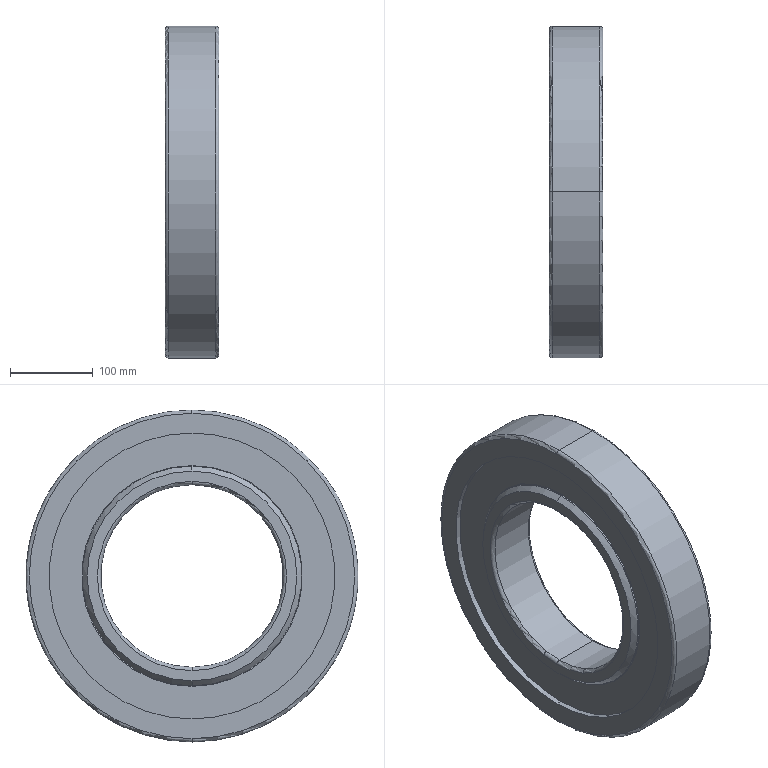Part | SolidWorks | features Revolution 5, Attribute 2, CirPattern 1, RefAxis 1 | 1 solid | 44 faces | box 65 x 400 x 400 mm | volume 5037424 mm3 | torus 16 | cylinder 16 | plane 8 | cone 4 | commonest cylinder face diameters 264.1 x4 344.425 x4 355.9 x4 220 x2 400 x2
STEP:
#1=CARTESIAN_POINT('',(32.5,0.,-126.312));
#2=VERTEX_POINT('',#1);
#3=CARTESIAN_POINT('',(32.5,0.,126.312));
#4=VERTEX_POINT('',#3);
#5=CARTESIAN_POINT('',(32.5,0.,0.));
#6=DIRECTION('',(1.,0.,0.));
#7=DIRECTION('',(0.,0.,-1.));
#8=AXIS2_PLACEMENT_3D('',#5,#6,#7);
#9=CIRCLE('',#8,126.313);
#10=EDGE_CURVE('',#2,#4,#9,.T.);
#11=ORIENTED_EDGE('',*,*,#10,.F.);
#12=CARTESIAN_POINT('',(26.,0.,-132.05));
#13=VERTEX_POINT('',#12);
#14=CARTESIAN_POINT('',(32.5,0.,-126.313));
#15=DIRECTION('',(-0.7497,0.,-0.6618));
#16=VECTOR('',#15,1000.);
#17=LINE('',#14,#16);
#18=EDGE_CURVE('',#2,#13,#17,.T.);
#19=ORIENTED_EDGE('',*,*,#18,.T.);
#20=CARTESIAN_POINT('',(26.,0.,132.05));
#21=VERTEX_POINT('',#20);
#22=CARTESIAN_POINT('',(26.,0.,0.));
#23=DIRECTION('',(1.,0.,0.));
#24=DIRECTION('',(0.,0.,-1.));
#25=AXIS2_PLACEMENT_3D('',#22,#23,#24);
#26=CIRCLE('',#25,132.05);
#27=EDGE_CURVE('',#13,#21,#26,.T.);
#28=ORIENTED_EDGE('',*,*,#27,.T.);
#29=CARTESIAN_POINT('',(32.5,0.,126.313));
#30=DIRECTION('',(-0.7497,0.,0.6618));
#31=VECTOR('',#30,1000.);
#32=LINE('',#29,#31);
#33=EDGE_CURVE('',#4,#21,#32,.T.);
#34=ORIENTED_EDGE('',*,*,#33,.F.);
#35=EDGE_LOOP('',(#11,#19,#28,#34));
#36=FACE_OUTER_BOUND('',#35,.T.);
#37=CARTESIAN_POINT('',(32.5,0.,0.));
#38=DIRECTION('',(-1.,0.,0.));
#39=DIRECTION('',(0.,0.,1.));
#40=AXIS2_PLACEMENT_3D('',#37,#38,#39);
#41=CONICAL_SURFACE('',#40,126.313,0.7232);
#42=ADVANCED_FACE('',(#36),#41,.T.);
#43=CARTESIAN_POINT('',(32.5,0.,-114.));
#44=VERTEX_POINT('',#43);
#45=CARTESIAN_POINT('',(32.5,0.,114.));
#46=VERTEX_POINT('',#45);
#47=CARTESIAN_POINT('',(32.5,0.,0.));
#48=DIRECTION('',(1.,0.,0.));
#49=DIRECTION('',(0.,0.,-1.));
#50=AXIS2_PLACEMENT_3D('',#47,#48,#49);
#51=CIRCLE('',#50,114.);
#52=EDGE_CURVE('',#44,#46,#51,.T.);
#53=ORIENTED_EDGE('',*,*,#52,.T.);
#54=CARTESIAN_POINT('',(28.5,0.,110.));
#55=VERTEX_POINT('',#54);
#56=CARTESIAN_POINT('',(28.5,0.,114.));
#57=DIRECTION('',(0.,1.,0.));
#58=DIRECTION('',(0.,0.,1.));
#59=AXIS2_PLACEMENT_3D('',#56,#57,#58);
#60=CIRCLE('',#59,4.);
#61=EDGE_CURVE('',#46,#55,#60,.T.);
#62=ORIENTED_EDGE('',*,*,#61,.T.);
#63=CARTESIAN_POINT('',(28.5,0.,-110.));
#64=VERTEX_POINT('',#63);
#65=CARTESIAN_POINT('',(28.5,0.,0.));
#66=DIRECTION('',(1.,0.,0.));
#67=DIRECTION('',(0.,0.,-1.));
#68=AXIS2_PLACEMENT_3D('',#65,#66,#67);
#69=CIRCLE('',#68,110.);
#70=EDGE_CURVE('',#64,#55,#69,.T.);
#71=ORIENTED_EDGE('',*,*,#70,.F.);
#72=CARTESIAN_POINT('',(28.5,0.,-114.));
#73=DIRECTION('',(0.,-1.,0.));
#74=DIRECTION('',(0.,0.,-1.));
#75=AXIS2_PLACEMENT_3D('',#72,#73,#74);
#76=CIRCLE('',#75,4.);
#77=EDGE_CURVE('',#44,#64,#76,.T.);
#78=ORIENTED_EDGE('',*,*,#77,.F.);
#79=EDGE_LOOP('',(#53,#62,#71,#78));
#80=FACE_OUTER_BOUND('',#79,.T.);
#81=CARTESIAN_POINT('',(28.5,0.,0.));
#82=DIRECTION('',(1.,0.,0.));
#83=DIRECTION('',(0.,0.,-1.));
#84=AXIS2_PLACEMENT_3D('',#81,#82,#83);
#85=TOROIDAL_SURFACE('',#84,114.,4.);
#86=ADVANCED_FACE('',(#80),#85,.T.);
#87=CARTESIAN_POINT('',(-28.5,0.,110.));
#88=VERTEX_POINT('',#87);
#89=CARTESIAN_POINT('',(-28.5,0.,-110.));
#90=VERTEX_POINT('',#89);
#91=CARTESIAN_POINT('',(-28.5,0.,0.));
#92=DIRECTION('',(1.,0.,0.));
#93=DIRECTION('',(0.,0.,-1.));
#94=AXIS2_PLACEMENT_3D('',#91,#92,#93);
#95=CIRCLE('',#94,110.);
#96=EDGE_CURVE('',#88,#90,#95,.T.);
#97=ORIENTED_EDGE('',*,*,#96,.F.);
#98=CARTESIAN_POINT('',(-90.,0.,110.));
#99=DIRECTION('',(1.,0.,0.));
#100=VECTOR('',#99,1000.);
#101=LINE('',#98,#100);
#102=EDGE_CURVE('',#88,#55,#101,.T.);
#103=ORIENTED_EDGE('',*,*,#102,.T.);
#104=CARTESIAN_POINT('',(28.5,0.,0.));
#105=DIRECTION('',(1.,0.,0.));
#106=DIRECTION('',(0.,0.,-1.));
#107=AXIS2_PLACEMENT_3D('',#104,#105,#106);
#108=CIRCLE('',#107,110.);
#109=EDGE_CURVE('',#55,#64,#108,.T.);
#110=ORIENTED_EDGE('',*,*,#109,.T.);
#111=CARTESIAN_POINT('',(-90.,0.,-110.));
#112=DIRECTION('',(1.,0.,0.));
#113=VECTOR('',#112,1000.);
#114=LINE('',#111,#113);
#115=EDGE_CURVE('',#90,#64,#114,.T.);
#116=ORIENTED_EDGE('',*,*,#115,.F.);
#117=EDGE_LOOP('',(#97,#103,#110,#116));
#118=FACE_OUTER_BOUND('',#117,.T.);
#119=CARTESIAN_POINT('',(-90.,0.,0.));
#120=DIRECTION('',(1.,0.,0.));
#121=DIRECTION('',(0.,0.,-1.));
#122=AXIS2_PLACEMENT_3D('',#119,#120,#121);
#123=CYLINDRICAL_SURFACE('',#122,110.);
#124=ADVANCED_FACE('',(#118),#123,.F.);
#125=CARTESIAN_POINT('',(-28.5,0.,0.));
#126=DIRECTION('',(1.,0.,0.));
#127=DIRECTION('',(0.,0.,-1.));
#128=AXIS2_PLACEMENT_3D('',#125,#126,#127);
#129=CIRCLE('',#128,110.);
#130=EDGE_CURVE('',#90,#88,#129,.T.);
#131=ORIENTED_EDGE('',*,*,#130,.T.);
#132=CARTESIAN_POINT('',(-32.5,0.,114.));
#133=VERTEX_POINT('',#132);
#134=CARTESIAN_POINT('',(-28.5,0.,114.));
#135=DIRECTION('',(0.,1.,0.));
#136=DIRECTION('',(0.,0.,1.));
#137=AXIS2_PLACEMENT_3D('',#134,#135,#136);
#138=CIRCLE('',#137,4.);
#139=EDGE_CURVE('',#88,#133,#138,.T.);
#140=ORIENTED_EDGE('',*,*,#139,.T.);
#141=CARTESIAN_POINT('',(-32.5,0.,-114.));
#142=VERTEX_POINT('',#141);
#143=CARTESIAN_POINT('',(-32.5,0.,0.));
#144=DIRECTION('',(1.,0.,0.));
#145=DIRECTION('',(0.,0.,-1.));
#146=AXIS2_PLACEMENT_3D('',#143,#144,#145);
#147=CIRCLE('',#146,114.);
#148=EDGE_CURVE('',#142,#133,#147,.T.);
#149=ORIENTED_EDGE('',*,*,#148,.F.);
#150=CARTESIAN_POINT('',(-28.5,0.,-114.));
#151=DIRECTION('',(0.,-1.,0.));
#152=DIRECTION('',(0.,0.,-1.));
#153=AXIS2_PLACEMENT_3D('',#150,#151,#152);
#154=CIRCLE('',#153,4.);
#155=EDGE_CURVE('',#90,#142,#154,.T.);
#156=ORIENTED_EDGE('',*,*,#155,.F.);
#157=EDGE_LOOP('',(#131,#140,#149,#156));
#158=FACE_OUTER_BOUND('',#157,.T.);
#159=CARTESIAN_POINT('',(-28.5,0.,0.));
#160=DIRECTION('',(1.,0.,0.));
#161=DIRECTION('',(0.,0.,-1.));
#162=AXIS2_PLACEMENT_3D('',#159,#160,#161);
#163=TOROIDAL_SURFACE('',#162,114.,4.);
#164=ADVANCED_FACE('',(#158),#163,.T.);
#165=CARTESIAN_POINT('',(-32.5,0.,-126.313));
#166=VERTEX_POINT('',#165);
#167=CARTESIAN_POINT('',(-32.5,0.,126.312));
#168=VERTEX_POINT('',#167);
#169=CARTESIAN_POINT('',(-32.5,0.,0.));
#170=DIRECTION('',(1.,0.,0.));
#171=DIRECTION('',(0.,0.,-1.));
#172=AXIS2_PLACEMENT_3D('',#169,#170,#171);
#173=CIRCLE('',#172,126.313);
#174=EDGE_CURVE('',#166,#168,#173,.T.);
#175=ORIENTED_EDGE('',*,*,#174,.T.);
#176=CARTESIAN_POINT('',(-26.,0.,132.05));
#177=VERTEX_POINT('',#176);
#178=CARTESIAN_POINT('',(-26.,0.,132.05));
#179=DIRECTION('',(0.7497,0.,0.6618));
#180=VECTOR('',#179,1000.);
#181=LINE('',#178,#180);
#182=EDGE_CURVE('',#168,#177,#181,.T.);
#183=ORIENTED_EDGE('',*,*,#182,.T.);
#184=CARTESIAN_POINT('',(-26.,0.,-132.05));
#185=VERTEX_POINT('',#184);
#186=CARTESIAN_POINT('',(-26.,0.,0.));
#187=DIRECTION('',(1.,0.,0.));
#188=DIRECTION('',(0.,0.,-1.));
#189=AXIS2_PLACEMENT_3D('',#186,#187,#188);
#190=CIRCLE('',#189,132.05);
#191=EDGE_CURVE('',#185,#177,#190,.T.);
#192=ORIENTED_EDGE('',*,*,#191,.F.);
#193=CARTESIAN_POINT('',(-26.,0.,-132.05));
#194=DIRECTION('',(0.7497,0.,-0.6618));
#195=VECTOR('',#194,1000.);
#196=LINE('',#193,#195);
#197=EDGE_CURVE('',#166,#185,#196,.T.);
#198=ORIENTED_EDGE('',*,*,#197,.F.);
#199=EDGE_LOOP('',(#175,#183,#192,#198));
#200=FACE_OUTER_BOUND('',#199,.T.);
#201=CARTESIAN_POINT('',(-26.,0.,0.));
#202=DIRECTION('',(1.,0.,0.));
#203=DIRECTION('',(0.,0.,-1.));
#204=AXIS2_PLACEMENT_3D('',#201,#202,#203);
#205=CONICAL_SURFACE('',#204,132.05,0.7232);
#206=ADVANCED_FACE('',(#200),#205,.T.);
#207=CARTESIAN_POINT('',(23.877,0.,-132.05));
#208=VERTEX_POINT('',#207);
#209=CARTESIAN_POINT('',(23.877,0.,132.05));
#210=VERTEX_POINT('',#209);
#211=CARTESIAN_POINT('',(23.877,0.,0.));
#212=DIRECTION('',(1.,0.,0.));
#213=DIRECTION('',(0.,0.,1.));
#214=AXIS2_PLACEMENT_3D('',#211,#212,#213);
#215=CIRCLE('',#214,132.05);
#216=EDGE_CURVE('',#208,#210,#215,.T.);
#217=ORIENTED_EDGE('',*,*,#216,.T.);
#218=CARTESIAN_POINT('',(-90.,0.,132.05));
#219=DIRECTION('',(1.,0.,0.));
#220=VECTOR('',#219,1000.);
#221=LINE('',#218,#220);
#222=EDGE_CURVE('',#210,#21,#221,.T.);
#223=ORIENTED_EDGE('',*,*,#222,.T.);
#224=ORIENTED_EDGE('',*,*,#27,.F.);
#225=CARTESIAN_POINT('',(-90.,0.,-132.05));
#226=DIRECTION('',(1.,0.,0.));
#227=VECTOR('',#226,1000.);
#228=LINE('',#225,#227);
#229=EDGE_CURVE('',#208,#13,#228,.T.);
#230=ORIENTED_EDGE('',*,*,#229,.F.);
#231=EDGE_LOOP('',(#217,#223,#224,#230));
#232=FACE_OUTER_BOUND('',#231,.T.);
#233=CARTESIAN_POINT('',(-90.,0.,0.));
#234=DIRECTION('',(1.,0.,0.));
#235=DIRECTION('',(0.,0.,-1.));
#236=AXIS2_PLACEMENT_3D('',#233,#234,#235);
#237=CYLINDRICAL_SURFACE('',#236,132.05);
#238=ADVANCED_FACE('',(#232),#237,.T.);
#239=ORIENTED_EDGE('',*,*,#191,.T.);
#240=CARTESIAN_POINT('',(-23.877,0.,132.05));
#241=VERTEX_POINT('',#240);
#242=CARTESIAN_POINT('',(-90.,0.,132.05));
#243=DIRECTION('',(1.,0.,0.));
#244=VECTOR('',#243,1000.);
#245=LINE('',#242,#244);
#246=EDGE_CURVE('',#177,#241,#245,.T.);
#247=ORIENTED_EDGE('',*,*,#246,.T.);
#248=CARTESIAN_POINT('',(-23.877,0.,-132.05));
#249=VERTEX_POINT('',#248);
#250=CARTESIAN_POINT('',(-23.877,0.,0.));
#251=DIRECTION('',(-1.,0.,0.));
#252=DIRECTION('',(0.,0.,-1.));
#253=AXIS2_PLACEMENT_3D('',#250,#251,#252);
#254=CIRCLE('',#253,132.05);
#255=EDGE_CURVE('',#241,#249,#254,.T.);
#256=ORIENTED_EDGE('',*,*,#255,.T.);
#257=CARTESIAN_POINT('',(-90.,0.,-132.05));
#258=DIRECTION('',(1.,0.,0.));
#259=VECTOR('',#258,1000.);
#260=LINE('',#257,#259);
#261=EDGE_CURVE('',#185,#249,#260,.T.);
#262=ORIENTED_EDGE('',*,*,#261,.F.);
#263=EDGE_LOOP('',(#239,#247,#256,#262));
#264=FACE_OUTER_BOUND('',#263,.T.);
#265=CARTESIAN_POINT('',(-90.,0.,0.));
#266=DIRECTION('',(1.,0.,0.));
#267=DIRECTION('',(0.,0.,-1.));
#268=AXIS2_PLACEMENT_3D('',#265,#266,#267);
#269=CYLINDRICAL_SURFACE('',#268,132.05);
#270=ADVANCED_FACE('',(#264),#269,.T.);
#271=CARTESIAN_POINT('',(23.877,0.,-177.95));
#272=VERTEX_POINT('',#271);
#273=CARTESIAN_POINT('',(23.877,0.,177.95));
#274=VERTEX_POINT('',#273);
#275=CARTESIAN_POINT('',(23.877,0.,0.));
#276=DIRECTION('',(1.,0.,0.));
#277=DIRECTION('',(0.,0.,1.));
#278=AXIS2_PLACEMENT_3D('',#275,#276,#277);
#279=CIRCLE('',#278,177.95);
#280=EDGE_CURVE('',#272,#274,#279,.T.);
#281=ORIENTED_EDGE('',*,*,#280,.T.);
#282=CARTESIAN_POINT('',(24.7,0.,177.037));
#283=VERTEX_POINT('',#282);
#284=CARTESIAN_POINT('',(23.782,0.,177.037));
#285=DIRECTION('',(0.,1.,0.));
#286=DIRECTION('',(0.,0.,1.));
#287=AXIS2_PLACEMENT_3D('',#284,#285,#286);
#288=CIRCLE('',#287,0.9182);
#289=EDGE_CURVE('',#274,#283,#288,.T.);
#290=ORIENTED_EDGE('',*,*,#289,.T.);
#291=CARTESIAN_POINT('',(24.7,0.,-177.037));
#292=VERTEX_POINT('',#291);
#293=CARTESIAN_POINT('',(24.7,0.,0.));
#294=DIRECTION('',(1.,0.,0.));
#295=DIRECTION('',(0.,0.,-1.));
#296=AXIS2_PLACEMENT_3D('',#293,#294,#295);
#297=CIRCLE('',#296,177.037);
#298=EDGE_CURVE('',#292,#283,#297,.T.);
#299=ORIENTED_EDGE('',*,*,#298,.F.);
#300=CARTESIAN_POINT('',(23.782,0.,-177.037));
#301=DIRECTION('',(0.,-1.,0.));
#302=DIRECTION('',(0.,0.,-1.));
#303=AXIS2_PLACEMENT_3D('',#300,#301,#302);
#304=CIRCLE('',#303,0.9182);
#305=EDGE_CURVE('',#272,#292,#304,.T.);
#306=ORIENTED_EDGE('',*,*,#305,.F.);
#307=EDGE_LOOP('',(#281,#290,#299,#306));
#308=FACE_OUTER_BOUND('',#307,.T.);
#309=CARTESIAN_POINT('',(23.782,0.,0.));
#310=DIRECTION('',(1.,0.,0.));
#311=DIRECTION('',(0.,0.,-1.));
#312=AXIS2_PLACEMENT_3D('',#309,#310,#311);
#313=TOROIDAL_SURFACE('',#312,177.037,0.9182);
#314=ADVANCED_FACE('',(#308),#313,.T.);
#315=CARTESIAN_POINT('',(24.7,0.,-132.963));
#316=VERTEX_POINT('',#315);
#317=CARTESIAN_POINT('',(24.7,0.,132.963));
#318=VERTEX_POINT('',#317);
#319=CARTESIAN_POINT('',(24.7,0.,0.));
#320=DIRECTION('',(1.,0.,0.));
#321=DIRECTION('',(0.,0.,-1.));
#322=AXIS2_PLACEMENT_3D('',#319,#320,#321);
#323=CIRCLE('',#322,132.963);
#324=EDGE_CURVE('',#316,#318,#323,.T.);
#325=ORIENTED_EDGE('',*,*,#324,.T.);
#326=CARTESIAN_POINT('',(23.782,0.,132.963));
#327=DIRECTION('',(0.,1.,0.));
#328=DIRECTION('',(0.,0.,1.));
#329=AXIS2_PLACEMENT_3D('',#326,#327,#328);
#330=CIRCLE('',#329,0.9182);
#331=EDGE_CURVE('',#318,#210,#330,.T.);
#332=ORIENTED_EDGE('',*,*,#331,.T.);
#333=ORIENTED_EDGE('',*,*,#216,.F.);
#334=CARTESIAN_POINT('',(23.782,0.,-132.963));
#335=DIRECTION('',(0.,-1.,0.));
#336=DIRECTION('',(0.,0.,-1.));
#337=AXIS2_PLACEMENT_3D('',#334,#335,#336);
#338=CIRCLE('',#337,0.9182);
#339=EDGE_CURVE('',#316,#208,#338,.T.);
#340=ORIENTED_EDGE('',*,*,#339,.F.);
#341=EDGE_LOOP('',(#325,#332,#333,#340));
#342=FACE_OUTER_BOUND('',#341,.T.);
#343=CARTESIAN_POINT('',(23.782,0.,0.));
#344=DIRECTION('',(1.,0.,0.));
#345=DIRECTION('',(0.,0.,-1.));
#346=AXIS2_PLACEMENT_3D('',#343,#344,#345);
#347=TOROIDAL_SURFACE('',#346,132.963,0.9182);
#348=ADVANCED_FACE('',(#342),#347,.T.);
#349=ORIENTED_EDGE('',*,*,#255,.F.);
#350=CARTESIAN_POINT('',(-24.7,0.,132.963));
#351=VERTEX_POINT('',#350);
#352=CARTESIAN_POINT('',(-23.782,0.,132.963));
#353=DIRECTION('',(0.,1.,0.));
#354=DIRECTION('',(0.,0.,1.));
#355=AXIS2_PLACEMENT_3D('',#352,#353,#354);
#356=CIRCLE('',#355,0.9182);
#357=EDGE_CURVE('',#241,#351,#356,.T.);
#358=ORIENTED_EDGE('',*,*,#357,.T.);
#359=CARTESIAN_POINT('',(-24.7,0.,-132.963));
#360=VERTEX_POINT('',#359);
#361=CARTESIAN_POINT('',(-24.7,0.,0.));
#362=DIRECTION('',(1.,0.,0.));
#363=DIRECTION('',(0.,0.,-1.));
#364=AXIS2_PLACEMENT_3D('',#361,#362,#363);
#365=CIRCLE('',#364,132.963);
#366=EDGE_CURVE('',#360,#351,#365,.T.);
#367=ORIENTED_EDGE('',*,*,#366,.F.);
#368=CARTESIAN_POINT('',(-23.782,0.,-132.963));
#369=DIRECTION('',(0.,-1.,0.));
#370=DIRECTION('',(0.,0.,-1.));
#371=AXIS2_PLACEMENT_3D('',#368,#369,#370);
#372=CIRCLE('',#371,0.9182);
#373=EDGE_CURVE('',#249,#360,#372,.T.);
#374=ORIENTED_EDGE('',*,*,#373,.F.);
#375=EDGE_LOOP('',(#349,#358,#367,#374));
#376=FACE_OUTER_BOUND('',#375,.T.);
#377=CARTESIAN_POINT('',(-23.782,0.,0.));
#378=DIRECTION('',(1.,0.,0.));
#379=DIRECTION('',(0.,0.,-1.));
#380=AXIS2_PLACEMENT_3D('',#377,#378,#379);
#381=TOROIDAL_SURFACE('',#380,132.963,0.9182);
#382=ADVANCED_FACE('',(#376),#381,.T.);
#383=CARTESIAN_POINT('',(-24.7,0.,-177.037));
#384=VERTEX_POINT('',#383);
#385=CARTESIAN_POINT('',(-24.7,0.,177.037));
#386=VERTEX_POINT('',#385);
#387=CARTESIAN_POINT('',(-24.7,0.,0.));
#388=DIRECTION('',(1.,0.,0.));
#389=DIRECTION('',(0.,0.,-1.));
#390=AXIS2_PLACEMENT_3D('',#387,#388,#389);
#391=CIRCLE('',#390,177.037);
#392=EDGE_CURVE('',#384,#386,#391,.T.);
#393=ORIENTED_EDGE('',*,*,#392,.T.);
#394=CARTESIAN_POINT('',(-23.877,0.,177.95));
#395=VERTEX_POINT('',#394);
#396=CARTESIAN_POINT('',(-23.782,0.,177.037));
#397=DIRECTION('',(0.,1.,0.));
#398=DIRECTION('',(0.,0.,1.));
#399=AXIS2_PLACEMENT_3D('',#396,#397,#398);
#400=CIRCLE('',#399,0.9182);
#401=EDGE_CURVE('',#386,#395,#400,.T.);
#402=ORIENTED_EDGE('',*,*,#401,.T.);
#403=CARTESIAN_POINT('',(-23.877,0.,-177.95));
#404=VERTEX_POINT('',#403);
#405=CARTESIAN_POINT('',(-23.877,0.,0.));
#406=DIRECTION('',(-1.,0.,0.));
#407=DIRECTION('',(0.,0.,-1.));
#408=AXIS2_PLACEMENT_3D('',#405,#406,#407);
#409=CIRCLE('',#408,177.95);
#410=EDGE_CURVE('',#395,#404,#409,.T.);
#411=ORIENTED_EDGE('',*,*,#410,.T.);
#412=CARTESIAN_POINT('',(-23.782,0.,-177.037));
#413=DIRECTION('',(0.,-1.,0.));
#414=DIRECTION('',(0.,0.,-1.));
#415=AXIS2_PLACEMENT_3D('',#412,#413,#414);
#416=CIRCLE('',#415,0.9182);
#417=EDGE_CURVE('',#384,#404,#416,.T.);
#418=ORIENTED_EDGE('',*,*,#417,.F.);
#419=EDGE_LOOP('',(#393,#402,#411,#418));
#420=FACE_OUTER_BOUND('',#419,.T.);
#421=CARTESIAN_POINT('',(-23.782,0.,0.));
#422=DIRECTION('',(1.,0.,0.));
#423=DIRECTION('',(0.,0.,-1.));
#424=AXIS2_PLACEMENT_3D('',#421,#422,#423);
#425=TOROIDAL_SURFACE('',#424,177.037,0.9182);
#426=ADVANCED_FACE('',(#420),#425,.T.);
#427=CARTESIAN_POINT('',(23.877,0.,0.));
#428=DIRECTION('',(1.,0.,0.));
#429=DIRECTION('',(0.,0.,1.));
#430=AXIS2_PLACEMENT_3D('',#427,#428,#429);
#431=CIRCLE('',#430,177.95);
#432=EDGE_CURVE('',#274,#272,#431,.T.);
#433=ORIENTED_EDGE('',*,*,#432,.F.);
#434=CARTESIAN_POINT('',(26.,0.,177.95));
#435=VERTEX_POINT('',#434);
#436=CARTESIAN_POINT('',(-90.,0.,177.95));
#437=DIRECTION('',(1.,0.,0.));
#438=VECTOR('',#437,1000.);
#439=LINE('',#436,#438);
#440=EDGE_CURVE('',#274,#435,#439,.T.);
#441=ORIENTED_EDGE('',*,*,#440,.T.);
#442=CARTESIAN_POINT('',(26.,0.,-177.95));
#443=VERTEX_POINT('',#442);
#444=CARTESIAN_POINT('',(26.,0.,0.));
#445=DIRECTION('',(1.,0.,0.));
#446=DIRECTION('',(0.,0.,-1.));
#447=AXIS2_PLACEMENT_3D('',#444,#445,#446);
#448=CIRCLE('',#447,177.95);
#449=EDGE_CURVE('',#435,#443,#448,.T.);
#450=ORIENTED_EDGE('',*,*,#449,.T.);
#451=CARTESIAN_POINT('',(-90.,0.,-177.95));
#452=DIRECTION('',(1.,0.,0.));
#453=VECTOR('',#452,1000.);
#454=LINE('',#451,#453);
#455=EDGE_CURVE('',#272,#443,#454,.T.);
#456=ORIENTED_EDGE('',*,*,#455,.F.);
#457=EDGE_LOOP('',(#433,#441,#450,#456));
#458=FACE_OUTER_BOUND('',#457,.T.);
#459=CARTESIAN_POINT('',(-90.,0.,0.));
#460=DIRECTION('',(1.,0.,0.));
#461=DIRECTION('',(0.,0.,-1.));
#462=AXIS2_PLACEMENT_3D('',#459,#460,#461);
#463=CYLINDRICAL_SURFACE('',#462,177.95);
#464=ADVANCED_FACE('',(#458),#463,.F.);
#465=CARTESIAN_POINT('',(26.,0.,172.213));
#466=VERTEX_POINT('',#465);
#467=CARTESIAN_POINT('',(26.,0.,-172.213));
#468=VERTEX_POINT('',#467);
#469=CARTESIAN_POINT('',(26.,0.,0.));
#470=DIRECTION('',(1.,0.,0.));
#471=DIRECTION('',(0.,0.,-1.));
#472=AXIS2_PLACEMENT_3D('',#469,#470,#471);
#473=CIRCLE('',#472,172.213);
#474=EDGE_CURVE('',#466,#468,#473,.T.);
#475=ORIENTED_EDGE('',*,*,#474,.F.);
#476=CARTESIAN_POINT('',(32.5,0.,172.213));
#477=VERTEX_POINT('',#476);
#478=CARTESIAN_POINT('',(-90.,0.,172.213));
#479=DIRECTION('',(1.,0.,0.));
#480=VECTOR('',#479,1000.);
#481=LINE('',#478,#480);
#482=EDGE_CURVE('',#466,#477,#481,.T.);
#483=ORIENTED_EDGE('',*,*,#482,.T.);
#484=CARTESIAN_POINT('',(32.5,0.,-172.213));
#485=VERTEX_POINT('',#484);
#486=CARTESIAN_POINT('',(32.5,0.,0.));
#487=DIRECTION('',(1.,0.,0.));
#488=DIRECTION('',(0.,0.,-1.));
#489=AXIS2_PLACEMENT_3D('',#486,#487,#488);
#490=CIRCLE('',#489,172.213);
#491=EDGE_CURVE('',#477,#485,#490,.T.);
#492=ORIENTED_EDGE('',*,*,#491,.T.);
#493=CARTESIAN_POINT('',(-90.,0.,-172.213));
#494=DIRECTION('',(1.,0.,0.));
#495=VECTOR('',#494,1000.);
#496=LINE('',#493,#495);
#497=EDGE_CURVE('',#468,#485,#496,.T.);
#498=ORIENTED_EDGE('',*,*,#497,.F.);
#499=EDGE_LOOP('',(#475,#483,#492,#498));
#500=FACE_OUTER_BOUND('',#499,.T.);
#501=CARTESIAN_POINT('',(-90.,0.,0.));
#502=DIRECTION('',(1.,0.,0.));
#503=DIRECTION('',(0.,0.,-1.));
#504=AXIS2_PLACEMENT_3D('',#501,#502,#503);
#505=CYLINDRICAL_SURFACE('',#504,172.213);
#506=ADVANCED_FACE('',(#500),#505,.F.);
#507=CARTESIAN_POINT('',(28.5,0.,-200.));
#508=VERTEX_POINT('',#507);
#509=CARTESIAN_POINT('',(28.5,0.,200.));
#510=VERTEX_POINT('',#509);
#511=CARTESIAN_POINT('',(28.5,0.,0.));
#512=DIRECTION('',(1.,0.,0.));
#513=DIRECTION('',(0.,0.,-1.));
#514=AXIS2_PLACEMENT_3D('',#511,#512,#513);
#515=CIRCLE('',#514,200.);
#516=EDGE_CURVE('',#508,#510,#515,.T.);
#517=ORIENTED_EDGE('',*,*,#516,.T.);
#518=CARTESIAN_POINT('',(32.5,0.,196.));
#519=VERTEX_POINT('',#518);
#520=CARTESIAN_POINT('',(28.5,0.,196.));
#521=DIRECTION('',(0.,1.,0.));
#522=DIRECTION('',(0.,0.,1.));
#523=AXIS2_PLACEMENT_3D('',#520,#521,#522);
#524=CIRCLE('',#523,4.);
#525=EDGE_CURVE('',#510,#519,#524,.T.);
#526=ORIENTED_EDGE('',*,*,#525,.T.);
#527=CARTESIAN_POINT('',(32.5,0.,-196.));
#528=VERTEX_POINT('',#527);
#529=CARTESIAN_POINT('',(32.5,0.,0.));
#530=DIRECTION('',(1.,0.,0.));
#531=DIRECTION('',(0.,0.,-1.));
#532=AXIS2_PLACEMENT_3D('',#529,#530,#531);
#533=CIRCLE('',#532,196.);
#534=EDGE_CURVE('',#528,#519,#533,.T.);
#535=ORIENTED_EDGE('',*,*,#534,.F.);
#536=CARTESIAN_POINT('',(28.5,0.,-196.));
#537=DIRECTION('',(0.,-1.,0.));
#538=DIRECTION('',(0.,0.,-1.));
#539=AXIS2_PLACEMENT_3D('',#536,#537,#538);
#540=CIRCLE('',#539,4.);
#541=EDGE_CURVE('',#508,#528,#540,.T.);
#542=ORIENTED_EDGE('',*,*,#541,.F.);
#543=EDGE_LOOP('',(#517,#526,#535,#542));
#544=FACE_OUTER_BOUND('',#543,.T.);
#545=CARTESIAN_POINT('',(28.5,0.,0.));
#546=DIRECTION('',(1.,0.,0.));
#547=DIRECTION('',(0.,0.,-1.));
#548=AXIS2_PLACEMENT_3D('',#545,#546,#547);
#549=TOROIDAL_SURFACE('',#548,196.,4.);
#550=ADVANCED_FACE('',(#544),#549,.T.);
#551=CARTESIAN_POINT('',(-28.5,0.,-200.));
#552=VERTEX_POINT('',#551);
#553=CARTESIAN_POINT('',(-28.5,0.,200.));
#554=VERTEX_POINT('',#553);
#555=CARTESIAN_POINT('',(-28.5,0.,0.));
#556=DIRECTION('',(1.,0.,0.));
#557=DIRECTION('',(0.,0.,-1.));
#558=AXIS2_PLACEMENT_3D('',#555,#556,#557);
#559=CIRCLE('',#558,200.);
#560=EDGE_CURVE('',#552,#554,#559,.T.);
#561=ORIENTED_EDGE('',*,*,#560,.T.);
#562=CARTESIAN_POINT('',(-90.,0.,200.));
#563=DIRECTION('',(1.,0.,0.));
#564=VECTOR('',#563,1000.);
#565=LINE('',#562,#564);
#566=EDGE_CURVE('',#554,#510,#565,.T.);
#567=ORIENTED_EDGE('',*,*,#566,.T.);
#568=ORIENTED_EDGE('',*,*,#516,.F.);
#569=CARTESIAN_POINT('',(-90.,0.,-200.));
#570=DIRECTION('',(1.,0.,0.));
#571=VECTOR('',#570,1000.);
#572=LINE('',#569,#571);
#573=EDGE_CURVE('',#552,#508,#572,.T.);
#574=ORIENTED_EDGE('',*,*,#573,.F.);
#575=EDGE_LOOP('',(#561,#567,#568,#574));
#576=FACE_OUTER_BOUND('',#575,.T.);
#577=CARTESIAN_POINT('',(-90.,0.,0.));
#578=DIRECTION('',(1.,0.,0.));
#579=DIRECTION('',(0.,0.,-1.));
#580=AXIS2_PLACEMENT_3D('',#577,#578,#579);
#581=CYLINDRICAL_SURFACE('',#580,200.);
#582=ADVANCED_FACE('',(#576),#581,.T.);
#583=CARTESIAN_POINT('',(-32.5,0.,-196.));
#584=VERTEX_POINT('',#583);
#585=CARTESIAN_POINT('',(-32.5,0.,196.));
#586=VERTEX_POINT('',#585);
#587=CARTESIAN_POINT('',(-32.5,0.,0.));
#588=DIRECTION('',(1.,0.,0.));
#589=DIRECTION('',(0.,0.,-1.));
#590=AXIS2_PLACEMENT_3D('',#587,#588,#589);
#591=CIRCLE('',#590,196.);
#592=EDGE_CURVE('',#584,#586,#591,.T.);
#593=ORIENTED_EDGE('',*,*,#592,.T.);
#594=CARTESIAN_POINT('',(-28.5,0.,196.));
#595=DIRECTION('',(0.,1.,0.));
#596=DIRECTION('',(0.,0.,1.));
#597=AXIS2_PLACEMENT_3D('',#594,#595,#596);
#598=CIRCLE('',#597,4.);
#599=EDGE_CURVE('',#586,#554,#598,.T.);
#600=ORIENTED_EDGE('',*,*,#599,.T.);
#601=ORIENTED_EDGE('',*,*,#560,.F.);
#602=CARTESIAN_POINT('',(-28.5,0.,-196.));
#603=DIRECTION('',(0.,-1.,0.));
#604=DIRECTION('',(0.,0.,-1.));
#605=AXIS2_PLACEMENT_3D('',#602,#603,#604);
#606=CIRCLE('',#605,4.);
#607=EDGE_CURVE('',#584,#552,#606,.T.);
#608=ORIENTED_EDGE('',*,*,#607,.F.);
#609=EDGE_LOOP('',(#593,#600,#601,#608));
#610=FACE_OUTER_BOUND('',#609,.T.);
#611=CARTESIAN_POINT('',(-28.5,0.,0.));
#612=DIRECTION('',(1.,0.,0.));
#613=DIRECTION('',(0.,0.,-1.));
#614=AXIS2_PLACEMENT_3D('',#611,#612,#613);
#615=TOROIDAL_SURFACE('',#614,196.,4.);
#616=ADVANCED_FACE('',(#610),#615,.T.);
#617=CARTESIAN_POINT('',(-32.5,0.,172.213));
#618=VERTEX_POINT('',#617);
#619=CARTESIAN_POINT('',(-32.5,0.,-172.213));
#620=VERTEX_POINT('',#619);
#621=CARTESIAN_POINT('',(-32.5,0.,0.));
#622=DIRECTION('',(1.,0.,0.));
#623=DIRECTION('',(0.,0.,-1.));
#624=AXIS2_PLACEMENT_3D('',#621,#622,#623);
#625=CIRCLE('',#624,172.213);
#626=EDGE_CURVE('',#618,#620,#625,.T.);
#627=ORIENTED_EDGE('',*,*,#626,.F.);
#628=CARTESIAN_POINT('',(-26.,0.,172.213));
#629=VERTEX_POINT('',#628);
#630=CARTESIAN_POINT('',(-90.,0.,172.213));
#631=DIRECTION('',(1.,0.,0.));
#632=VECTOR('',#631,1000.);
#633=LINE('',#630,#632);
#634=EDGE_CURVE('',#618,#629,#633,.T.);
#635=ORIENTED_EDGE('',*,*,#634,.T.);
#636=CARTESIAN_POINT('',(-26.,0.,-172.213));
#637=VERTEX_POINT('',#636);
#638=CARTESIAN_POINT('',(-26.,0.,0.));
#639=DIRECTION('',(1.,0.,0.));
#640=DIRECTION('',(0.,0.,-1.));
#641=AXIS2_PLACEMENT_3D('',#638,#639,#640);
#642=CIRCLE('',#641,172.213);
#643=EDGE_CURVE('',#629,#637,#642,.T.);
#644=ORIENTED_EDGE('',*,*,#643,.T.);
#645=CARTESIAN_POINT('',(-90.,0.,-172.213));
#646=DIRECTION('',(1.,0.,0.));
#647=VECTOR('',#646,1000.);
#648=LINE('',#645,#647);
#649=EDGE_CURVE('',#620,#637,#648,.T.);
#650=ORIENTED_EDGE('',*,*,#649,.F.);
#651=EDGE_LOOP('',(#627,#635,#644,#650));
#652=FACE_OUTER_BOUND('',#651,.T.);
#653=CARTESIAN_POINT('',(-90.,0.,0.));
#654=DIRECTION('',(1.,0.,0.));
#655=DIRECTION('',(0.,0.,-1.));
#656=AXIS2_PLACEMENT_3D('',#653,#654,#655);
#657=CYLINDRICAL_SURFACE('',#656,172.213);
#658=ADVANCED_FACE('',(#652),#657,.F.);
#659=CARTESIAN_POINT('',(-26.,0.,177.95));
#660=VERTEX_POINT('',#659);
#661=CARTESIAN_POINT('',(-26.,0.,-177.95));
#662=VERTEX_POINT('',#661);
#663=CARTESIAN_POINT('',(-26.,0.,0.));
#664=DIRECTION('',(1.,0.,0.));
#665=DIRECTION('',(0.,0.,-1.));
#666=AXIS2_PLACEMENT_3D('',#663,#664,#665);
#667=CIRCLE('',#666,177.95);
#668=EDGE_CURVE('',#660,#662,#667,.T.);
#669=ORIENTED_EDGE('',*,*,#668,.F.);
#670=CARTESIAN_POINT('',(-90.,0.,177.95));
#671=DIRECTION('',(1.,0.,0.));
#672=VECTOR('',#671,1000.);
#673=LINE('',#670,#672);
#674=EDGE_CURVE('',#660,#395,#673,.T.);
#675=ORIENTED_EDGE('',*,*,#674,.T.);
#676=CARTESIAN_POINT('',(-23.877,0.,0.));
#677=DIRECTION('',(-1.,0.,0.));
#678=DIRECTION('',(0.,0.,-1.));
#679=AXIS2_PLACEMENT_3D('',#676,#677,#678);
#680=CIRCLE('',#679,177.95);
#681=EDGE_CURVE('',#404,#395,#680,.T.);
#682=ORIENTED_EDGE('',*,*,#681,.F.);
#683=CARTESIAN_POINT('',(-90.,0.,-177.95));
#684=DIRECTION('',(1.,0.,0.));
#685=VECTOR('',#684,1000.);
#686=LINE('',#683,#685);
#687=EDGE_CURVE('',#662,#404,#686,.T.);
#688=ORIENTED_EDGE('',*,*,#687,.F.);
#689=EDGE_LOOP('',(#669,#675,#682,#688));
#690=FACE_OUTER_BOUND('',#689,.T.);
#691=CARTESIAN_POINT('',(-90.,0.,0.));
#692=DIRECTION('',(1.,0.,0.));
#693=DIRECTION('',(0.,0.,-1.));
#694=AXIS2_PLACEMENT_3D('',#691,#692,#693);
#695=CYLINDRICAL_SURFACE('',#694,177.95);
#696=ADVANCED_FACE('',(#690),#695,.F.);
#697=ORIENTED_EDGE('',*,*,#674,.F.);
#698=CARTESIAN_POINT('',(-26.,0.,0.));
#699=DIRECTION('',(1.,0.,0.));
#700=DIRECTION('',(0.,0.,-1.));
#701=AXIS2_PLACEMENT_3D('',#698,#699,#700);
#702=CIRCLE('',#701,177.95);
#703=EDGE_CURVE('',#662,#660,#702,.T.);
#704=ORIENTED_EDGE('',*,*,#703,.F.);
#705=ORIENTED_EDGE('',*,*,#687,.T.);
#706=ORIENTED_EDGE('',*,*,#410,.F.);
#707=EDGE_LOOP('',(#697,#704,#705,#706));
#708=FACE_OUTER_BOUND('',#707,.T.);
#709=CARTESIAN_POINT('',(-90.,0.,0.));
#710=DIRECTION('',(1.,0.,0.));
#711=DIRECTION('',(0.,0.,-1.));
#712=AXIS2_PLACEMENT_3D('',#709,#710,#711);
#713=CYLINDRICAL_SURFACE('',#712,177.95);
#714=ADVANCED_FACE('',(#708),#713,.F.);
#715=ORIENTED_EDGE('',*,*,#703,.T.);
#716=ORIENTED_EDGE('',*,*,#668,.T.);
#717=EDGE_LOOP('',(#715,#716));
#718=FACE_OUTER_BOUND('',#717,.T.);
#719=CARTESIAN_POINT('',(-26.,0.,0.));
#720=DIRECTION('',(1.,0.,0.));
#721=DIRECTION('',(0.,0.,-1.));
#722=AXIS2_PLACEMENT_3D('',#719,#720,#721);
#723=CIRCLE('',#722,172.213);
#724=EDGE_CURVE('',#637,#629,#723,.T.);
#725=ORIENTED_EDGE('',*,*,#724,.F.);
#726=ORIENTED_EDGE('',*,*,#643,.F.);
#727=EDGE_LOOP('',(#725,#726));
#728=FACE_BOUND('',#727,.T.);
#729=CARTESIAN_POINT('',(-26.,177.95,0.));
#730=DIRECTION('',(1.,0.,0.));
#731=DIRECTION('',(0.,0.,-1.));
#732=AXIS2_PLACEMENT_3D('',#729,#730,#731);
#733=PLANE('',#732);
#734=ADVANCED_FACE('',(#718,#728),#733,.T.);
#735=ORIENTED_EDGE('',*,*,#634,.F.);
#736=CARTESIAN_POINT('',(-32.5,0.,0.));
#737=DIRECTION('',(1.,0.,0.));
#738=DIRECTION('',(0.,0.,-1.));
#739=AXIS2_PLACEMENT_3D('',#736,#737,#738);
#740=CIRCLE('',#739,172.213);
#741=EDGE_CURVE('',#620,#618,#740,.T.);
#742=ORIENTED_EDGE('',*,*,#741,.F.);
#743=ORIENTED_EDGE('',*,*,#649,.T.);
#744=ORIENTED_EDGE('',*,*,#724,.T.);
#745=EDGE_LOOP('',(#735,#742,#743,#744));
#746=FACE_OUTER_BOUND('',#745,.T.);
#747=CARTESIAN_POINT('',(-90.,0.,0.));
#748=DIRECTION('',(1.,0.,0.));
#749=DIRECTION('',(0.,0.,-1.));
#750=AXIS2_PLACEMENT_3D('',#747,#748,#749);
#751=CYLINDRICAL_SURFACE('',#750,172.213);
#752=ADVANCED_FACE('',(#746),#751,.F.);
#753=ORIENTED_EDGE('',*,*,#741,.T.);
#754=ORIENTED_EDGE('',*,*,#626,.T.);
#755=EDGE_LOOP('',(#753,#754));
#756=FACE_BOUND('',#755,.T.);
#757=ORIENTED_EDGE('',*,*,#592,.F.);
#758=CARTESIAN_POINT('',(-32.5,0.,0.));
#759=DIRECTION('',(1.,0.,0.));
#760=DIRECTION('',(0.,0.,-1.));
#761=AXIS2_PLACEMENT_3D('',#758,#759,#760);
#762=CIRCLE('',#761,196.);
#763=EDGE_CURVE('',#586,#584,#762,.T.);
#764=ORIENTED_EDGE('',*,*,#763,.F.);
#765=EDGE_LOOP('',(#757,#764));
#766=FACE_OUTER_BOUND('',#765,.T.);
#767=CARTESIAN_POINT('',(-32.5,172.213,0.));
#768=DIRECTION('',(-1.,0.,0.));
#769=DIRECTION('',(0.,0.,1.));
#770=AXIS2_PLACEMENT_3D('',#767,#768,#769);
#771=PLANE('',#770);
#772=ADVANCED_FACE('',(#756,#766),#771,.T.);
#773=ORIENTED_EDGE('',*,*,#599,.F.);
#774=ORIENTED_EDGE('',*,*,#763,.T.);
#775=ORIENTED_EDGE('',*,*,#607,.T.);
#776=CARTESIAN_POINT('',(-28.5,0.,0.));
#777=DIRECTION('',(1.,0.,0.));
#778=DIRECTION('',(0.,0.,-1.));
#779=AXIS2_PLACEMENT_3D('',#776,#777,#778);
#780=CIRCLE('',#779,200.);
#781=EDGE_CURVE('',#554,#552,#780,.T.);
#782=ORIENTED_EDGE('',*,*,#781,.F.);
#783=EDGE_LOOP('',(#773,#774,#775,#782));
#784=FACE_OUTER_BOUND('',#783,.T.);
#785=CARTESIAN_POINT('',(-28.5,0.,0.));
#786=DIRECTION('',(1.,0.,0.));
#787=DIRECTION('',(0.,0.,-1.));
#788=AXIS2_PLACEMENT_3D('',#785,#786,#787);
#789=TOROIDAL_SURFACE('',#788,196.,4.);
#790=ADVANCED_FACE('',(#784),#789,.T.);
#791=ORIENTED_EDGE('',*,*,#566,.F.);
#792=ORIENTED_EDGE('',*,*,#781,.T.);
#793=ORIENTED_EDGE('',*,*,#573,.T.);
#794=CARTESIAN_POINT('',(28.5,0.,0.));
#795=DIRECTION('',(1.,0.,0.));
#796=DIRECTION('',(0.,0.,-1.));
#797=AXIS2_PLACEMENT_3D('',#794,#795,#796);
#798=CIRCLE('',#797,200.);
#799=EDGE_CURVE('',#510,#508,#798,.T.);
#800=ORIENTED_EDGE('',*,*,#799,.F.);
#801=EDGE_LOOP('',(#791,#792,#793,#800));
#802=FACE_OUTER_BOUND('',#801,.T.);
#803=CARTESIAN_POINT('',(-90.,0.,0.));
#804=DIRECTION('',(1.,0.,0.));
#805=DIRECTION('',(0.,0.,-1.));
#806=AXIS2_PLACEMENT_3D('',#803,#804,#805);
#807=CYLINDRICAL_SURFACE('',#806,200.);
#808=ADVANCED_FACE('',(#802),#807,.T.);
#809=ORIENTED_EDGE('',*,*,#525,.F.);
#810=ORIENTED_EDGE('',*,*,#799,.T.);
#811=ORIENTED_EDGE('',*,*,#541,.T.);
#812=CARTESIAN_POINT('',(32.5,0.,0.));
#813=DIRECTION('',(1.,0.,0.));
#814=DIRECTION('',(0.,0.,-1.));
#815=AXIS2_PLACEMENT_3D('',#812,#813,#814);
#816=CIRCLE('',#815,196.);
#817=EDGE_CURVE('',#519,#528,#816,.T.);
#818=ORIENTED_EDGE('',*,*,#817,.F.);
#819=EDGE_LOOP('',(#809,#810,#811,#818));
#820=FACE_OUTER_BOUND('',#819,.T.);
#821=CARTESIAN_POINT('',(28.5,0.,0.));
#822=DIRECTION('',(1.,0.,0.));
#823=DIRECTION('',(0.,0.,-1.));
#824=AXIS2_PLACEMENT_3D('',#821,#822,#823);
#825=TOROIDAL_SURFACE('',#824,196.,4.);
#826=ADVANCED_FACE('',(#820),#825,.T.);
#827=ORIENTED_EDGE('',*,*,#534,.T.);
#828=ORIENTED_EDGE('',*,*,#817,.T.);
#829=EDGE_LOOP('',(#827,#828));
#830=FACE_OUTER_BOUND('',#829,.T.);
#831=CARTESIAN_POINT('',(32.5,0.,0.));
#832=DIRECTION('',(1.,0.,0.));
#833=DIRECTION('',(0.,0.,-1.));
#834=AXIS2_PLACEMENT_3D('',#831,#832,#833);
#835=CIRCLE('',#834,172.213);
#836=EDGE_CURVE('',#485,#477,#835,.T.);
#837=ORIENTED_EDGE('',*,*,#836,.F.);
#838=ORIENTED_EDGE('',*,*,#491,.F.);
#839=EDGE_LOOP('',(#837,#838));
#840=FACE_BOUND('',#839,.T.);
#841=CARTESIAN_POINT('',(32.5,196.,0.));
#842=DIRECTION('',(1.,0.,0.));
#843=DIRECTION('',(0.,0.,-1.));
#844=AXIS2_PLACEMENT_3D('',#841,#842,#843);
#845=PLANE('',#844);
#846=ADVANCED_FACE('',(#830,#840),#845,.T.);
#847=ORIENTED_EDGE('',*,*,#482,.F.);
#848=CARTESIAN_POINT('',(26.,0.,0.));
#849=DIRECTION('',(1.,0.,0.));
#850=DIRECTION('',(0.,0.,-1.));
#851=AXIS2_PLACEMENT_3D('',#848,#849,#850);
#852=CIRCLE('',#851,172.213);
#853=EDGE_CURVE('',#468,#466,#852,.T.);
#854=ORIENTED_EDGE('',*,*,#853,.F.);
#855=ORIENTED_EDGE('',*,*,#497,.T.);
#856=ORIENTED_EDGE('',*,*,#836,.T.);
#857=EDGE_LOOP('',(#847,#854,#855,#856));
#858=FACE_OUTER_BOUND('',#857,.T.);
#859=CARTESIAN_POINT('',(-90.,0.,0.));
#860=DIRECTION('',(1.,0.,0.));
#861=DIRECTION('',(0.,0.,-1.));
#862=AXIS2_PLACEMENT_3D('',#859,#860,#861);
#863=CYLINDRICAL_SURFACE('',#862,172.213);
#864=ADVANCED_FACE('',(#858),#863,.F.);
#865=ORIENTED_EDGE('',*,*,#853,.T.);
#866=ORIENTED_EDGE('',*,*,#474,.T.);
#867=EDGE_LOOP('',(#865,#866));
#868=FACE_BOUND('',#867,.T.);
#869=CARTESIAN_POINT('',(26.,0.,0.));
#870=DIRECTION('',(1.,0.,0.));
#871=DIRECTION('',(0.,0.,-1.));
#872=AXIS2_PLACEMENT_3D('',#869,#870,#871);
#873=CIRCLE('',#872,177.95);
#874=EDGE_CURVE('',#443,#435,#873,.T.);
#875=ORIENTED_EDGE('',*,*,#874,.F.);
#876=ORIENTED_EDGE('',*,*,#449,.F.);
#877=EDGE_LOOP('',(#875,#876));
#878=FACE_OUTER_BOUND('',#877,.T.);
#879=CARTESIAN_POINT('',(26.,172.213,0.));
#880=DIRECTION('',(-1.,0.,0.));
#881=DIRECTION('',(0.,0.,1.));
#882=AXIS2_PLACEMENT_3D('',#879,#880,#881);
#883=PLANE('',#882);
#884=ADVANCED_FACE('',(#868,#878),#883,.T.);
#885=ORIENTED_EDGE('',*,*,#440,.F.);
#886=ORIENTED_EDGE('',*,*,#280,.F.);
#887=ORIENTED_EDGE('',*,*,#455,.T.);
#888=ORIENTED_EDGE('',*,*,#874,.T.);
#889=EDGE_LOOP('',(#885,#886,#887,#888));
#890=FACE_OUTER_BOUND('',#889,.T.);
#891=CARTESIAN_POINT('',(-90.,0.,0.));
#892=DIRECTION('',(1.,0.,0.));
#893=DIRECTION('',(0.,0.,-1.));
#894=AXIS2_PLACEMENT_3D('',#891,#892,#893);
#895=CYLINDRICAL_SURFACE('',#894,177.95);
#896=ADVANCED_FACE('',(#890),#895,.F.);
#897=ORIENTED_EDGE('',*,*,#401,.F.);
#898=CARTESIAN_POINT('',(-24.7,0.,0.));
#899=DIRECTION('',(1.,0.,0.));
#900=DIRECTION('',(0.,0.,-1.));
#901=AXIS2_PLACEMENT_3D('',#898,#899,#900);
#902=CIRCLE('',#901,177.037);
#903=EDGE_CURVE('',#386,#384,#902,.T.);
#904=ORIENTED_EDGE('',*,*,#903,.T.);
#905=ORIENTED_EDGE('',*,*,#417,.T.);
#906=ORIENTED_EDGE('',*,*,#681,.T.);
#907=EDGE_LOOP('',(#897,#904,#905,#906));
#908=FACE_OUTER_BOUND('',#907,.T.);
#909=CARTESIAN_POINT('',(-23.782,0.,0.));
#910=DIRECTION('',(1.,0.,0.));
#911=DIRECTION('',(0.,0.,-1.));
#912=AXIS2_PLACEMENT_3D('',#909,#910,#911);
#913=TOROIDAL_SURFACE('',#912,177.037,0.9182);
#914=ADVANCED_FACE('',(#908),#913,.T.);
#915=ORIENTED_EDGE('',*,*,#366,.T.);
#916=CARTESIAN_POINT('',(-24.7,0.,0.));
#917=DIRECTION('',(1.,0.,0.));
#918=DIRECTION('',(0.,0.,-1.));
#919=AXIS2_PLACEMENT_3D('',#916,#917,#918);
#920=CIRCLE('',#919,132.963);
#921=EDGE_CURVE('',#351,#360,#920,.T.);
#922=ORIENTED_EDGE('',*,*,#921,.T.);
#923=EDGE_LOOP('',(#915,#922));
#924=FACE_BOUND('',#923,.T.);
#925=ORIENTED_EDGE('',*,*,#392,.F.);
#926=ORIENTED_EDGE('',*,*,#903,.F.);
#927=EDGE_LOOP('',(#925,#926));
#928=FACE_OUTER_BOUND('',#927,.T.);
#929=CARTESIAN_POINT('',(-24.7,177.037,0.));
#930=DIRECTION('',(-1.,0.,0.));
#931=DIRECTION('',(0.,0.,1.));
#932=AXIS2_PLACEMENT_3D('',#929,#930,#931);
#933=PLANE('',#932);
#934=ADVANCED_FACE('',(#924,#928),#933,.T.);
#935=ORIENTED_EDGE('',*,*,#357,.F.);
#936=CARTESIAN_POINT('',(-23.877,0.,0.));
#937=DIRECTION('',(-1.,0.,0.));
#938=DIRECTION('',(0.,0.,-1.));
#939=AXIS2_PLACEMENT_3D('',#936,#937,#938);
#940=CIRCLE('',#939,132.05);
#941=EDGE_CURVE('',#249,#241,#940,.T.);
#942=ORIENTED_EDGE('',*,*,#941,.F.);
#943=ORIENTED_EDGE('',*,*,#373,.T.);
#944=ORIENTED_EDGE('',*,*,#921,.F.);
#945=EDGE_LOOP('',(#935,#942,#943,#944));
#946=FACE_OUTER_BOUND('',#945,.T.);
#947=CARTESIAN_POINT('',(-23.782,0.,0.));
#948=DIRECTION('',(1.,0.,0.));
#949=DIRECTION('',(0.,0.,-1.));
#950=AXIS2_PLACEMENT_3D('',#947,#948,#949);
#951=TOROIDAL_SURFACE('',#950,132.963,0.9182);
#952=ADVANCED_FACE('',(#946),#951,.T.);
#953=ORIENTED_EDGE('',*,*,#331,.F.);
#954=CARTESIAN_POINT('',(24.7,0.,0.));
#955=DIRECTION('',(1.,0.,0.));
#956=DIRECTION('',(0.,0.,-1.));
#957=AXIS2_PLACEMENT_3D('',#954,#955,#956);
#958=CIRCLE('',#957,132.963);
#959=EDGE_CURVE('',#318,#316,#958,.T.);
#960=ORIENTED_EDGE('',*,*,#959,.T.);
#961=ORIENTED_EDGE('',*,*,#339,.T.);
#962=CARTESIAN_POINT('',(23.877,0.,0.));
#963=DIRECTION('',(1.,0.,0.));
#964=DIRECTION('',(0.,0.,1.));
#965=AXIS2_PLACEMENT_3D('',#962,#963,#964);
#966=CIRCLE('',#965,132.05);
#967=EDGE_CURVE('',#210,#208,#966,.T.);
#968=ORIENTED_EDGE('',*,*,#967,.F.);
#969=EDGE_LOOP('',(#953,#960,#961,#968));
#970=FACE_OUTER_BOUND('',#969,.T.);
#971=CARTESIAN_POINT('',(23.782,0.,0.));
#972=DIRECTION('',(1.,0.,0.));
#973=DIRECTION('',(0.,0.,-1.));
#974=AXIS2_PLACEMENT_3D('',#971,#972,#973);
#975=TOROIDAL_SURFACE('',#974,132.963,0.9182);
#976=ADVANCED_FACE('',(#970),#975,.T.);
#977=ORIENTED_EDGE('',*,*,#298,.T.);
#978=CARTESIAN_POINT('',(24.7,0.,0.));
#979=DIRECTION('',(1.,0.,0.));
#980=DIRECTION('',(0.,0.,-1.));
#981=AXIS2_PLACEMENT_3D('',#978,#979,#980);
#982=CIRCLE('',#981,177.037);
#983=EDGE_CURVE('',#283,#292,#982,.T.);
#984=ORIENTED_EDGE('',*,*,#983,.T.);
#985=EDGE_LOOP('',(#977,#984));
#986=FACE_OUTER_BOUND('',#985,.T.);
#987=ORIENTED_EDGE('',*,*,#324,.F.);
#988=ORIENTED_EDGE('',*,*,#959,.F.);
#989=EDGE_LOOP('',(#987,#988));
#990=FACE_BOUND('',#989,.T.);
#991=CARTESIAN_POINT('',(24.7,132.963,0.));
#992=DIRECTION('',(1.,0.,0.));
#993=DIRECTION('',(0.,0.,-1.));
#994=AXIS2_PLACEMENT_3D('',#991,#992,#993);
#995=PLANE('',#994);
#996=ADVANCED_FACE('',(#986,#990),#995,.T.);
#997=ORIENTED_EDGE('',*,*,#289,.F.);
#998=ORIENTED_EDGE('',*,*,#432,.T.);
#999=ORIENTED_EDGE('',*,*,#305,.T.);
#1000=ORIENTED_EDGE('',*,*,#983,.F.);
#1001=EDGE_LOOP('',(#997,#998,#999,#1000));
#1002=FACE_OUTER_BOUND('',#1001,.T.);
#1003=CARTESIAN_POINT('',(23.782,0.,0.));
#1004=DIRECTION('',(1.,0.,0.));
#1005=DIRECTION('',(0.,0.,-1.));
#1006=AXIS2_PLACEMENT_3D('',#1003,#1004,#1005);
#1007=TOROIDAL_SURFACE('',#1006,177.037,0.9182);
#1008=ADVANCED_FACE('',(#1002),#1007,.T.);
#1009=ORIENTED_EDGE('',*,*,#246,.F.);
#1010=CARTESIAN_POINT('',(-26.,0.,0.));
#1011=DIRECTION('',(1.,0.,0.));
#1012=DIRECTION('',(0.,0.,-1.));
#1013=AXIS2_PLACEMENT_3D('',#1010,#1011,#1012);
#1014=CIRCLE('',#1013,132.05);
#1015=EDGE_CURVE('',#177,#185,#1014,.T.);
#1016=ORIENTED_EDGE('',*,*,#1015,.T.);
#1017=ORIENTED_EDGE('',*,*,#261,.T.);
#1018=ORIENTED_EDGE('',*,*,#941,.T.);
#1019=EDGE_LOOP('',(#1009,#1016,#1017,#1018));
#1020=FACE_OUTER_BOUND('',#1019,.T.);
#1021=CARTESIAN_POINT('',(-90.,0.,0.));
#1022=DIRECTION('',(1.,0.,0.));
#1023=DIRECTION('',(0.,0.,-1.));
#1024=AXIS2_PLACEMENT_3D('',#1021,#1022,#1023);
#1025=CYLINDRICAL_SURFACE('',#1024,132.05);
#1026=ADVANCED_FACE('',(#1020),#1025,.T.);
#1027=ORIENTED_EDGE('',*,*,#222,.F.);
#1028=ORIENTED_EDGE('',*,*,#967,.T.);
#1029=ORIENTED_EDGE('',*,*,#229,.T.);
#1030=CARTESIAN_POINT('',(26.,0.,0.));
#1031=DIRECTION('',(1.,0.,0.));
#1032=DIRECTION('',(0.,0.,-1.));
#1033=AXIS2_PLACEMENT_3D('',#1030,#1031,#1032);
#1034=CIRCLE('',#1033,132.05);
#1035=EDGE_CURVE('',#21,#13,#1034,.T.);
#1036=ORIENTED_EDGE('',*,*,#1035,.F.);
#1037=EDGE_LOOP('',(#1027,#1028,#1029,#1036));
#1038=FACE_OUTER_BOUND('',#1037,.T.);
#1039=CARTESIAN_POINT('',(-90.,0.,0.));
#1040=DIRECTION('',(1.,0.,0.));
#1041=DIRECTION('',(0.,0.,-1.));
#1042=AXIS2_PLACEMENT_3D('',#1039,#1040,#1041);
#1043=CYLINDRICAL_SURFACE('',#1042,132.05);
#1044=ADVANCED_FACE('',(#1038),#1043,.T.);
#1045=ORIENTED_EDGE('',*,*,#182,.F.);
#1046=CARTESIAN_POINT('',(-32.5,0.,0.));
#1047=DIRECTION('',(1.,0.,0.));
#1048=DIRECTION('',(0.,0.,-1.));
#1049=AXIS2_PLACEMENT_3D('',#1046,#1047,#1048);
#1050=CIRCLE('',#1049,126.313);
#1051=EDGE_CURVE('',#168,#166,#1050,.T.);
#1052=ORIENTED_EDGE('',*,*,#1051,.T.);
#1053=ORIENTED_EDGE('',*,*,#197,.T.);
#1054=ORIENTED_EDGE('',*,*,#1015,.F.);
#1055=EDGE_LOOP('',(#1045,#1052,#1053,#1054));
#1056=FACE_OUTER_BOUND('',#1055,.T.);
#1057=CARTESIAN_POINT('',(-26.,0.,0.));
#1058=DIRECTION('',(1.,0.,0.));
#1059=DIRECTION('',(0.,0.,-1.));
#1060=AXIS2_PLACEMENT_3D('',#1057,#1058,#1059);
#1061=CONICAL_SURFACE('',#1060,132.05,0.7232);
#1062=ADVANCED_FACE('',(#1056),#1061,.T.);
#1063=ORIENTED_EDGE('',*,*,#148,.T.);
#1064=CARTESIAN_POINT('',(-32.5,0.,0.));
#1065=DIRECTION('',(1.,0.,0.));
#1066=DIRECTION('',(0.,0.,-1.));
#1067=AXIS2_PLACEMENT_3D('',#1064,#1065,#1066);
#1068=CIRCLE('',#1067,114.);
#1069=EDGE_CURVE('',#133,#142,#1068,.T.);
#1070=ORIENTED_EDGE('',*,*,#1069,.T.);
#1071=EDGE_LOOP('',(#1063,#1070));
#1072=FACE_BOUND('',#1071,.T.);
#1073=ORIENTED_EDGE('',*,*,#174,.F.);
#1074=ORIENTED_EDGE('',*,*,#1051,.F.);
#1075=EDGE_LOOP('',(#1073,#1074));
#1076=FACE_OUTER_BOUND('',#1075,.T.);
#1077=CARTESIAN_POINT('',(-32.5,126.313,0.));
#1078=DIRECTION('',(-1.,0.,0.));
#1079=DIRECTION('',(0.,0.,1.));
#1080=AXIS2_PLACEMENT_3D('',#1077,#1078,#1079);
#1081=PLANE('',#1080);
#1082=ADVANCED_FACE('',(#1072,#1076),#1081,.T.);
#1083=ORIENTED_EDGE('',*,*,#139,.F.);
#1084=ORIENTED_EDGE('',*,*,#96,.T.);
#1085=ORIENTED_EDGE('',*,*,#155,.T.);
#1086=ORIENTED_EDGE('',*,*,#1069,.F.);
#1087=EDGE_LOOP('',(#1083,#1084,#1085,#1086));
#1088=FACE_OUTER_BOUND('',#1087,.T.);
#1089=CARTESIAN_POINT('',(-28.5,0.,0.));
#1090=DIRECTION('',(1.,0.,0.));
#1091=DIRECTION('',(0.,0.,-1.));
#1092=AXIS2_PLACEMENT_3D('',#1089,#1090,#1091);
#1093=TOROIDAL_SURFACE('',#1092,114.,4.);
#1094=ADVANCED_FACE('',(#1088),#1093,.T.);
#1095=ORIENTED_EDGE('',*,*,#102,.F.);
#1096=ORIENTED_EDGE('',*,*,#130,.F.);
#1097=ORIENTED_EDGE('',*,*,#115,.T.);
#1098=ORIENTED_EDGE('',*,*,#70,.T.);
#1099=EDGE_LOOP('',(#1095,#1096,#1097,#1098));
#1100=FACE_OUTER_BOUND('',#1099,.T.);
#1101=CARTESIAN_POINT('',(-90.,0.,0.));
#1102=DIRECTION('',(1.,0.,0.));
#1103=DIRECTION('',(0.,0.,-1.));
#1104=AXIS2_PLACEMENT_3D('',#1101,#1102,#1103);
#1105=CYLINDRICAL_SURFACE('',#1104,110.);
#1106=ADVANCED_FACE('',(#1100),#1105,.F.);
#1107=ORIENTED_EDGE('',*,*,#61,.F.);
#1108=CARTESIAN_POINT('',(32.5,0.,0.));
#1109=DIRECTION('',(1.,0.,0.));
#1110=DIRECTION('',(0.,0.,-1.));
#1111=AXIS2_PLACEMENT_3D('',#1108,#1109,#1110);
#1112=CIRCLE('',#1111,114.);
#1113=EDGE_CURVE('',#46,#44,#1112,.T.);
#1114=ORIENTED_EDGE('',*,*,#1113,.T.);
#1115=ORIENTED_EDGE('',*,*,#77,.T.);
#1116=ORIENTED_EDGE('',*,*,#109,.F.);
#1117=EDGE_LOOP('',(#1107,#1114,#1115,#1116));
#1118=FACE_OUTER_BOUND('',#1117,.T.);
#1119=CARTESIAN_POINT('',(28.5,0.,0.));
#1120=DIRECTION('',(1.,0.,0.));
#1121=DIRECTION('',(0.,0.,-1.));
#1122=AXIS2_PLACEMENT_3D('',#1119,#1120,#1121);
#1123=TOROIDAL_SURFACE('',#1122,114.,4.);
#1124=ADVANCED_FACE('',(#1118),#1123,.T.);
#1125=CARTESIAN_POINT('',(32.5,0.,0.));
#1126=DIRECTION('',(1.,0.,0.));
#1127=DIRECTION('',(0.,0.,-1.));
#1128=AXIS2_PLACEMENT_3D('',#1125,#1126,#1127);
#1129=CIRCLE('',#1128,126.313);
#1130=EDGE_CURVE('',#4,#2,#1129,.T.);
#1131=ORIENTED_EDGE('',*,*,#1130,.T.);
#1132=ORIENTED_EDGE('',*,*,#10,.T.);
#1133=EDGE_LOOP('',(#1131,#1132));
#1134=FACE_OUTER_BOUND('',#1133,.T.);
#1135=ORIENTED_EDGE('',*,*,#52,.F.);
#1136=ORIENTED_EDGE('',*,*,#1113,.F.);
#1137=EDGE_LOOP('',(#1135,#1136));
#1138=FACE_BOUND('',#1137,.T.);
#1139=CARTESIAN_POINT('',(32.5,114.,0.));
#1140=DIRECTION('',(1.,0.,0.));
#1141=DIRECTION('',(0.,0.,-1.));
#1142=AXIS2_PLACEMENT_3D('',#1139,#1140,#1141);
#1143=PLANE('',#1142);
#1144=ADVANCED_FACE('',(#1134,#1138),#1143,.T.);
#1145=ORIENTED_EDGE('',*,*,#18,.F.);
#1146=ORIENTED_EDGE('',*,*,#1130,.F.);
#1147=ORIENTED_EDGE('',*,*,#33,.T.);
#1148=ORIENTED_EDGE('',*,*,#1035,.T.);
#1149=EDGE_LOOP('',(#1145,#1146,#1147,#1148));
#1150=FACE_OUTER_BOUND('',#1149,.T.);
#1151=CARTESIAN_POINT('',(32.5,0.,0.));
#1152=DIRECTION('',(-1.,0.,0.));
#1153=DIRECTION('',(0.,0.,1.));
#1154=AXIS2_PLACEMENT_3D('',#1151,#1152,#1153);
#1155=CONICAL_SURFACE('',#1154,126.313,0.7232);
#1156=ADVANCED_FACE('',(#1150),#1155,.T.);
#1157=CLOSED_SHELL('',(#42,#86,#124,#164,#206,#238,#270,#314,#348,#382,#426,#464,#506,#550,#582,#616,#658,#696,#714,#734,#752,#772,#790,#808,#826,#846,#864,#884,#896,#914,#934,#952,#976,#996,#1008,#1026,#1044,#1062,#1082,#1094,#1106,#1124,#1144,#1156));
#1158=MANIFOLD_SOLID_BREP('',#1157);
#1159=CARTESIAN_POINT('',(0.,0.,0.));
#1160=DIRECTION('',(0.,0.,1.));
#1161=DIRECTION('',(1.,0.,0.));
#1162=AXIS2_PLACEMENT_3D('',#1159,#1160,#1161);
#1163=(LENGTH_UNIT()NAMED_UNIT(*)SI_UNIT(.MILLI.,.METRE.));
#1164=UNCERTAINTY_MEASURE_WITH_UNIT(LENGTH_MEASURE(0.00001),#1163,'','');
#1165=(NAMED_UNIT(*)PLANE_ANGLE_UNIT()SI_UNIT($,.RADIAN.));
#1166=(NAMED_UNIT(*)SI_UNIT($,.STERADIAN.)SOLID_ANGLE_UNIT());
#1167=(GEOMETRIC_REPRESENTATION_CONTEXT(3)GLOBAL_UNCERTAINTY_ASSIGNED_CONTEXT((#1164))GLOBAL_UNIT_ASSIGNED_CONTEXT((#1163,#1165,#1166))REPRESENTATION_CONTEXT('',''));
#1168=ADVANCED_BREP_SHAPE_REPRESENTATION('',(#1158,#1162),#1167);